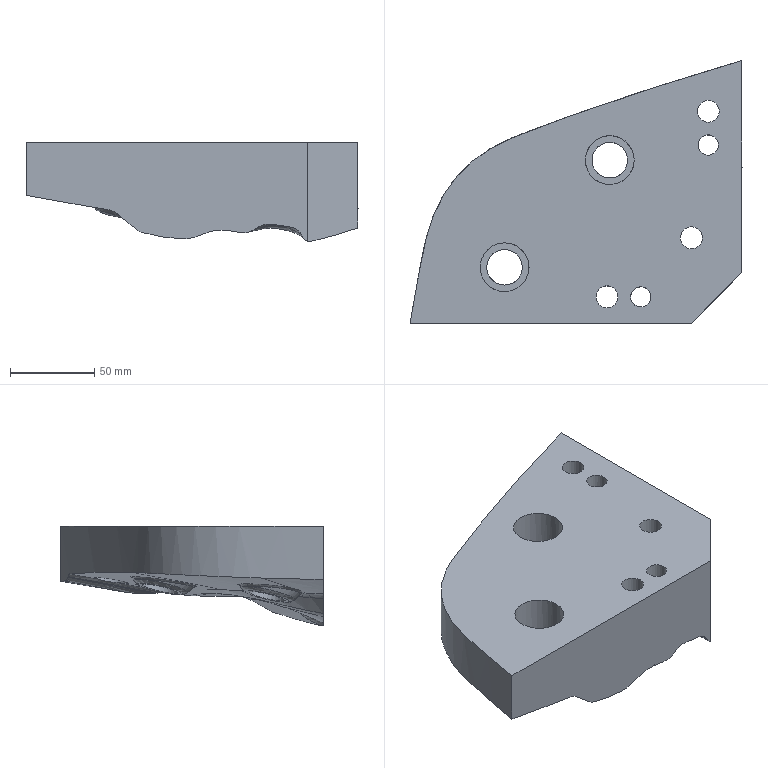Part | NX | features solid 2 | 1 solid | 81 faces | box 196.771 x 155.578 x 59.061 mm | volume 764350 mm3 | spline 60 | cylinder 12 | plane 9 | commonest cylinder face diameters 13 x3 20 x3 12 x2 21.1 x2 29 x2